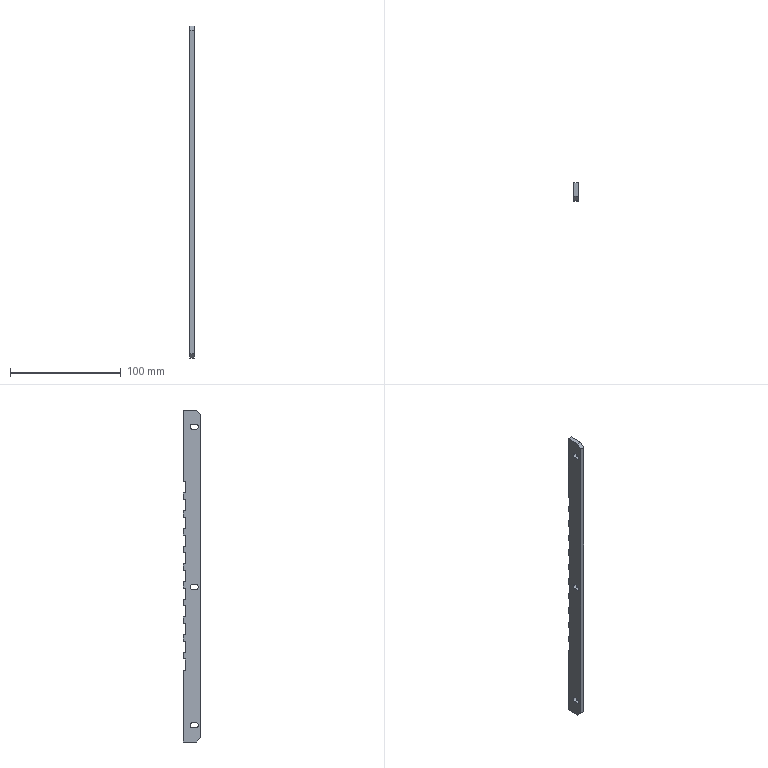Part | SolidWorks | features ICE 3, Chamfer 1, Extrusion 1, LPattern 1, MirrorPattern 1 | 1 solid | 64 faces | box 4 x 16 x 300 mm | volume 17903 mm3 | plane 58 | cylinder 6 | commonest cylinder face diameters 4.5 x6